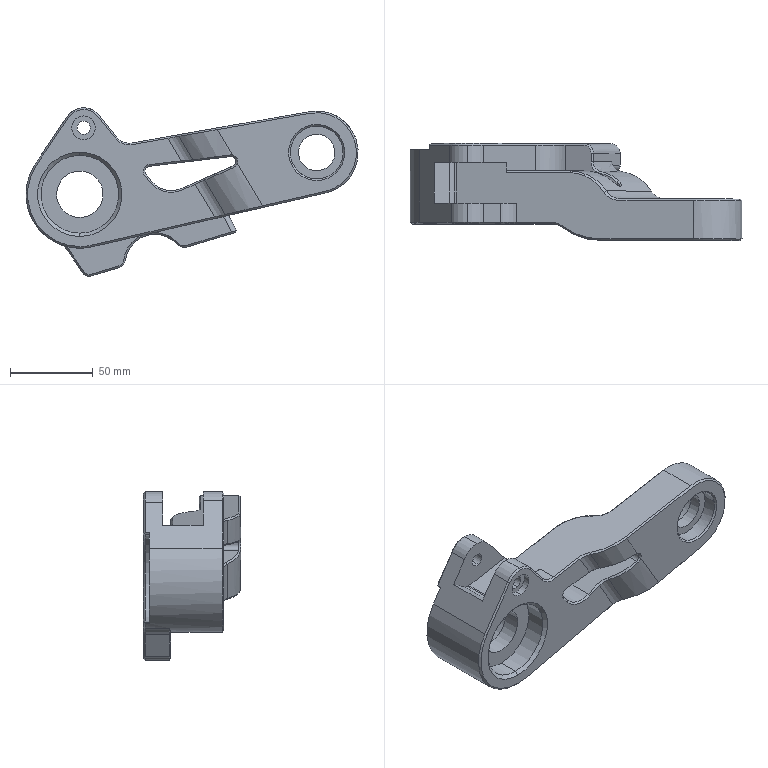Part | SolidWorks | features BaseBody 1 | 1 solid | 173 faces | box 200.297 x 58.5 x 101.592 mm | volume 315687 mm3 | plane 60 | cylinder 52 | cone 38 | spline 23 | commonest cylinder face diameters 10 x7 20 x5 5 x4 7.95 x4 14.2 x4 24 x4